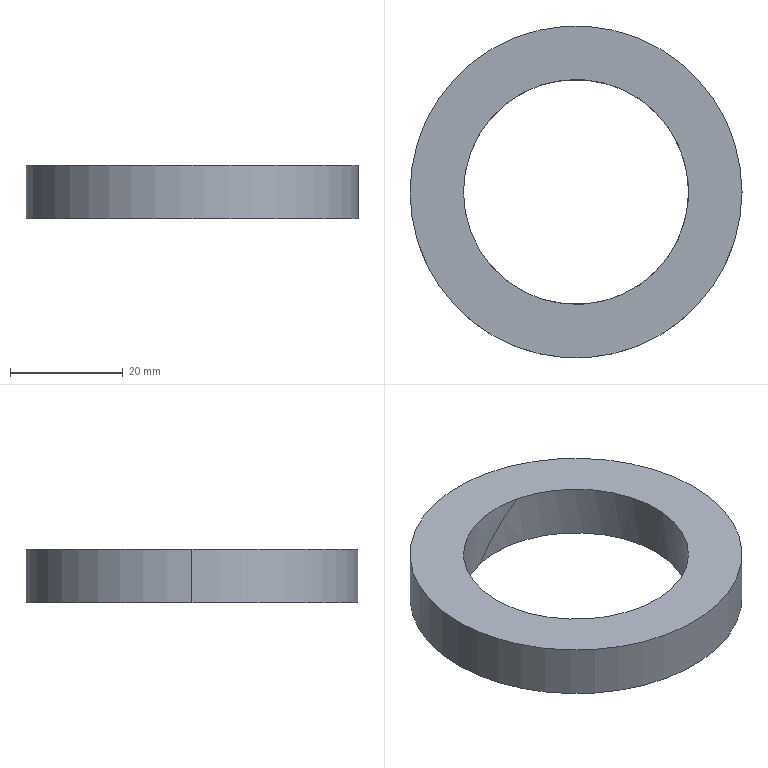Part | SolidWorks | features Extrusion 1, PLine 1 | 1 solid | 7 faces | box 59 x 59 x 9.5 mm | volume 14035 mm3 | cylinder 5 | plane 2 | commonest cylinder face diameters 40 x3 59 x2
STEP:
#1=CARTESIAN_POINT('',(29.5,0.,9.5));
#2=VERTEX_POINT('',#1);
#3=CARTESIAN_POINT('',(-29.5,0.,9.5));
#4=VERTEX_POINT('',#3);
#5=CARTESIAN_POINT('',(0.,0.,9.5));
#6=DIRECTION('',(0.,0.,1.));
#7=DIRECTION('',(1.,0.,0.));
#8=AXIS2_PLACEMENT_3D('',#5,#6,#7);
#9=CIRCLE('',#8,29.5);
#10=EDGE_CURVE('',#2,#4,#9,.T.);
#11=ORIENTED_EDGE('',*,*,#10,.F.);
#12=CARTESIAN_POINT('',(29.5,0.,0.));
#13=VERTEX_POINT('',#12);
#14=CARTESIAN_POINT('',(29.5,0.,9.5));
#15=DIRECTION('',(0.,0.,-1.));
#16=VECTOR('',#15,1000.);
#17=LINE('',#14,#16);
#18=EDGE_CURVE('',#2,#13,#17,.T.);
#19=ORIENTED_EDGE('',*,*,#18,.T.);
#20=CARTESIAN_POINT('',(-29.5,0.,0.));
#21=VERTEX_POINT('',#20);
#22=CARTESIAN_POINT('',(0.,0.,0.));
#23=DIRECTION('',(0.,0.,1.));
#24=DIRECTION('',(1.,0.,0.));
#25=AXIS2_PLACEMENT_3D('',#22,#23,#24);
#26=CIRCLE('',#25,29.5);
#27=EDGE_CURVE('',#13,#21,#26,.T.);
#28=ORIENTED_EDGE('',*,*,#27,.T.);
#29=CARTESIAN_POINT('',(-29.5,0.,9.5));
#30=DIRECTION('',(0.,0.,-1.));
#31=VECTOR('',#30,1000.);
#32=LINE('',#29,#31);
#33=EDGE_CURVE('',#4,#21,#32,.T.);
#34=ORIENTED_EDGE('',*,*,#33,.F.);
#35=EDGE_LOOP('',(#11,#19,#28,#34));
#36=FACE_OUTER_BOUND('',#35,.T.);
#37=CARTESIAN_POINT('',(0.,0.,9.5));
#38=DIRECTION('',(0.,0.,-1.));
#39=DIRECTION('',(-1.,0.,0.));
#40=AXIS2_PLACEMENT_3D('',#37,#38,#39);
#41=CYLINDRICAL_SURFACE('',#40,29.5);
#42=ADVANCED_FACE('',(#36),#41,.T.);
#43=CARTESIAN_POINT('',(4.75,19.428,9.5));
#44=VERTEX_POINT('',#43);
#45=CARTESIAN_POINT('',(-20.,0.,9.5));
#46=VERTEX_POINT('',#45);
#47=CARTESIAN_POINT('',(0.,0.,9.5));
#48=DIRECTION('',(0.,0.,1.));
#49=DIRECTION('',(1.,0.,0.));
#50=AXIS2_PLACEMENT_3D('',#47,#48,#49);
#51=CIRCLE('',#50,20.);
#52=EDGE_CURVE('',#44,#46,#51,.T.);
#53=ORIENTED_EDGE('',*,*,#52,.T.);
#54=CARTESIAN_POINT('',(-20.,0.,0.));
#55=VERTEX_POINT('',#54);
#56=CARTESIAN_POINT('',(-20.,0.,9.5));
#57=DIRECTION('',(0.,0.,-1.));
#58=VECTOR('',#57,1000.);
#59=LINE('',#56,#58);
#60=EDGE_CURVE('',#46,#55,#59,.T.);
#61=ORIENTED_EDGE('',*,*,#60,.T.);
#62=CARTESIAN_POINT('',(-4.75,19.428,0.));
#63=VERTEX_POINT('',#62);
#64=CARTESIAN_POINT('',(0.,0.,0.));
#65=DIRECTION('',(0.,0.,1.));
#66=DIRECTION('',(1.,0.,0.));
#67=AXIS2_PLACEMENT_3D('',#64,#65,#66);
#68=CIRCLE('',#67,20.);
#69=EDGE_CURVE('',#63,#55,#68,.T.);
#70=ORIENTED_EDGE('',*,*,#69,.F.);
#71=CARTESIAN_POINT('',(-4.75,19.428,0.));
#72=CARTESIAN_POINT('',(-1.614,20.194,3.136));
#73=CARTESIAN_POINT('',(1.614,20.194,6.364));
#74=CARTESIAN_POINT('',(4.75,19.428,9.5));
#75=(BOUNDED_CURVE()B_SPLINE_CURVE(3,(#71,#72,#73,#74),.UNSPECIFIED.,.F.,.T.)B_SPLINE_CURVE_WITH_KNOTS((4,4),(1.331,1.811),.UNSPECIFIED.)CURVE()GEOMETRIC_REPRESENTATION_ITEM()RATIONAL_B_SPLINE_CURVE((1.,0.9809,0.9809,1.))REPRESENTATION_ITEM(''));
#76=EDGE_CURVE('',#63,#44,#75,.T.);
#77=ORIENTED_EDGE('',*,*,#76,.T.);
#78=EDGE_LOOP('',(#53,#61,#70,#77));
#79=FACE_OUTER_BOUND('',#78,.T.);
#80=CARTESIAN_POINT('',(0.,0.,9.5));
#81=DIRECTION('',(0.,0.,-1.));
#82=DIRECTION('',(-1.,0.,0.));
#83=AXIS2_PLACEMENT_3D('',#80,#81,#82);
#84=CYLINDRICAL_SURFACE('',#83,20.);
#85=ADVANCED_FACE('',(#79),#84,.F.);
#86=ORIENTED_EDGE('',*,*,#60,.F.);
#87=CARTESIAN_POINT('',(4.75,-19.428,9.5));
#88=VERTEX_POINT('',#87);
#89=CARTESIAN_POINT('',(0.,0.,9.5));
#90=DIRECTION('',(0.,0.,1.));
#91=DIRECTION('',(1.,0.,0.));
#92=AXIS2_PLACEMENT_3D('',#89,#90,#91);
#93=CIRCLE('',#92,20.);
#94=EDGE_CURVE('',#46,#88,#93,.T.);
#95=ORIENTED_EDGE('',*,*,#94,.T.);
#96=CARTESIAN_POINT('',(-4.75,-19.428,0.));
#97=VERTEX_POINT('',#96);
#98=CARTESIAN_POINT('',(4.75,-19.428,9.5));
#99=CARTESIAN_POINT('',(1.614,-20.194,6.364));
#100=CARTESIAN_POINT('',(-1.614,-20.194,3.136));
#101=CARTESIAN_POINT('',(-4.75,-19.428,0.));
#102=(BOUNDED_CURVE()B_SPLINE_CURVE(3,(#98,#99,#100,#101),.UNSPECIFIED.,.F.,.F.)B_SPLINE_CURVE_WITH_KNOTS((4,4),(4.473,4.952),.UNSPECIFIED.)CURVE()GEOMETRIC_REPRESENTATION_ITEM()RATIONAL_B_SPLINE_CURVE((1.,0.9809,0.9809,1.))REPRESENTATION_ITEM(''));
#103=EDGE_CURVE('',#88,#97,#102,.T.);
#104=ORIENTED_EDGE('',*,*,#103,.T.);
#105=CARTESIAN_POINT('',(0.,0.,0.));
#106=DIRECTION('',(0.,0.,1.));
#107=DIRECTION('',(1.,0.,0.));
#108=AXIS2_PLACEMENT_3D('',#105,#106,#107);
#109=CIRCLE('',#108,20.);
#110=EDGE_CURVE('',#55,#97,#109,.T.);
#111=ORIENTED_EDGE('',*,*,#110,.F.);
#112=EDGE_LOOP('',(#86,#95,#104,#111));
#113=FACE_OUTER_BOUND('',#112,.T.);
#114=CARTESIAN_POINT('',(0.,0.,9.5));
#115=DIRECTION('',(0.,0.,-1.));
#116=DIRECTION('',(-1.,0.,0.));
#117=AXIS2_PLACEMENT_3D('',#114,#115,#116);
#118=CYLINDRICAL_SURFACE('',#117,20.);
#119=ADVANCED_FACE('',(#113),#118,.F.);
#120=CARTESIAN_POINT('',(0.,0.,9.5));
#121=DIRECTION('',(0.,0.,1.));
#122=DIRECTION('',(1.,0.,0.));
#123=AXIS2_PLACEMENT_3D('',#120,#121,#122);
#124=CIRCLE('',#123,29.5);
#125=EDGE_CURVE('',#4,#2,#124,.T.);
#126=ORIENTED_EDGE('',*,*,#125,.T.);
#127=ORIENTED_EDGE('',*,*,#10,.T.);
#128=EDGE_LOOP('',(#126,#127));
#129=FACE_OUTER_BOUND('',#128,.T.);
#130=ORIENTED_EDGE('',*,*,#52,.F.);
#131=CARTESIAN_POINT('',(0.,0.,9.5));
#132=DIRECTION('',(0.,0.,1.));
#133=DIRECTION('',(1.,0.,0.));
#134=AXIS2_PLACEMENT_3D('',#131,#132,#133);
#135=CIRCLE('',#134,20.);
#136=EDGE_CURVE('',#88,#44,#135,.T.);
#137=ORIENTED_EDGE('',*,*,#136,.F.);
#138=ORIENTED_EDGE('',*,*,#94,.F.);
#139=EDGE_LOOP('',(#130,#137,#138));
#140=FACE_BOUND('',#139,.T.);
#141=CARTESIAN_POINT('',(0.,0.,9.5));
#142=DIRECTION('',(0.,0.,1.));
#143=DIRECTION('',(1.,0.,0.));
#144=AXIS2_PLACEMENT_3D('',#141,#142,#143);
#145=PLANE('',#144);
#146=ADVANCED_FACE('',(#129,#140),#145,.T.);
#147=CARTESIAN_POINT('',(0.,0.,0.));
#148=DIRECTION('',(0.,0.,1.));
#149=DIRECTION('',(1.,0.,0.));
#150=AXIS2_PLACEMENT_3D('',#147,#148,#149);
#151=CIRCLE('',#150,29.5);
#152=EDGE_CURVE('',#21,#13,#151,.T.);
#153=ORIENTED_EDGE('',*,*,#152,.F.);
#154=ORIENTED_EDGE('',*,*,#27,.F.);
#155=EDGE_LOOP('',(#153,#154));
#156=FACE_OUTER_BOUND('',#155,.T.);
#157=ORIENTED_EDGE('',*,*,#69,.T.);
#158=ORIENTED_EDGE('',*,*,#110,.T.);
#159=CARTESIAN_POINT('',(0.,0.,0.));
#160=DIRECTION('',(0.,0.,1.));
#161=DIRECTION('',(1.,0.,0.));
#162=AXIS2_PLACEMENT_3D('',#159,#160,#161);
#163=CIRCLE('',#162,20.);
#164=EDGE_CURVE('',#97,#63,#163,.T.);
#165=ORIENTED_EDGE('',*,*,#164,.T.);
#166=EDGE_LOOP('',(#157,#158,#165));
#167=FACE_BOUND('',#166,.T.);
#168=CARTESIAN_POINT('',(0.,0.,0.));
#169=DIRECTION('',(0.,0.,1.));
#170=DIRECTION('',(1.,0.,0.));
#171=AXIS2_PLACEMENT_3D('',#168,#169,#170);
#172=PLANE('',#171);
#173=ADVANCED_FACE('',(#156,#167),#172,.F.);
#174=ORIENTED_EDGE('',*,*,#18,.F.);
#175=ORIENTED_EDGE('',*,*,#125,.F.);
#176=ORIENTED_EDGE('',*,*,#33,.T.);
#177=ORIENTED_EDGE('',*,*,#152,.T.);
#178=EDGE_LOOP('',(#174,#175,#176,#177));
#179=FACE_OUTER_BOUND('',#178,.T.);
#180=CARTESIAN_POINT('',(0.,0.,9.5));
#181=DIRECTION('',(0.,0.,-1.));
#182=DIRECTION('',(-1.,0.,0.));
#183=AXIS2_PLACEMENT_3D('',#180,#181,#182);
#184=CYLINDRICAL_SURFACE('',#183,29.5);
#185=ADVANCED_FACE('',(#179),#184,.T.);
#186=ORIENTED_EDGE('',*,*,#76,.F.);
#187=ORIENTED_EDGE('',*,*,#164,.F.);
#188=ORIENTED_EDGE('',*,*,#103,.F.);
#189=ORIENTED_EDGE('',*,*,#136,.T.);
#190=EDGE_LOOP('',(#186,#187,#188,#189));
#191=FACE_OUTER_BOUND('',#190,.T.);
#192=CARTESIAN_POINT('',(0.,0.,9.5));
#193=DIRECTION('',(0.,0.,-1.));
#194=DIRECTION('',(-1.,0.,0.));
#195=AXIS2_PLACEMENT_3D('',#192,#193,#194);
#196=CYLINDRICAL_SURFACE('',#195,20.);
#197=ADVANCED_FACE('',(#191),#196,.F.);
#198=CLOSED_SHELL('',(#42,#85,#119,#146,#173,#185,#197));
#199=MANIFOLD_SOLID_BREP('',#198);
#200=CARTESIAN_POINT('',(0.,0.,0.));
#201=DIRECTION('',(0.,0.,1.));
#202=DIRECTION('',(1.,0.,0.));
#203=AXIS2_PLACEMENT_3D('',#200,#201,#202);
#204=(LENGTH_UNIT()NAMED_UNIT(*)SI_UNIT(.MILLI.,.METRE.));
#205=UNCERTAINTY_MEASURE_WITH_UNIT(LENGTH_MEASURE(0.00001),#204,'','');
#206=(NAMED_UNIT(*)PLANE_ANGLE_UNIT()SI_UNIT($,.RADIAN.));
#207=(NAMED_UNIT(*)SI_UNIT($,.STERADIAN.)SOLID_ANGLE_UNIT());
#208=(GEOMETRIC_REPRESENTATION_CONTEXT(3)GLOBAL_UNCERTAINTY_ASSIGNED_CONTEXT((#205))GLOBAL_UNIT_ASSIGNED_CONTEXT((#204,#206,#207))REPRESENTATION_CONTEXT('',''));
#209=ADVANCED_BREP_SHAPE_REPRESENTATION('',(#199,#203),#208);